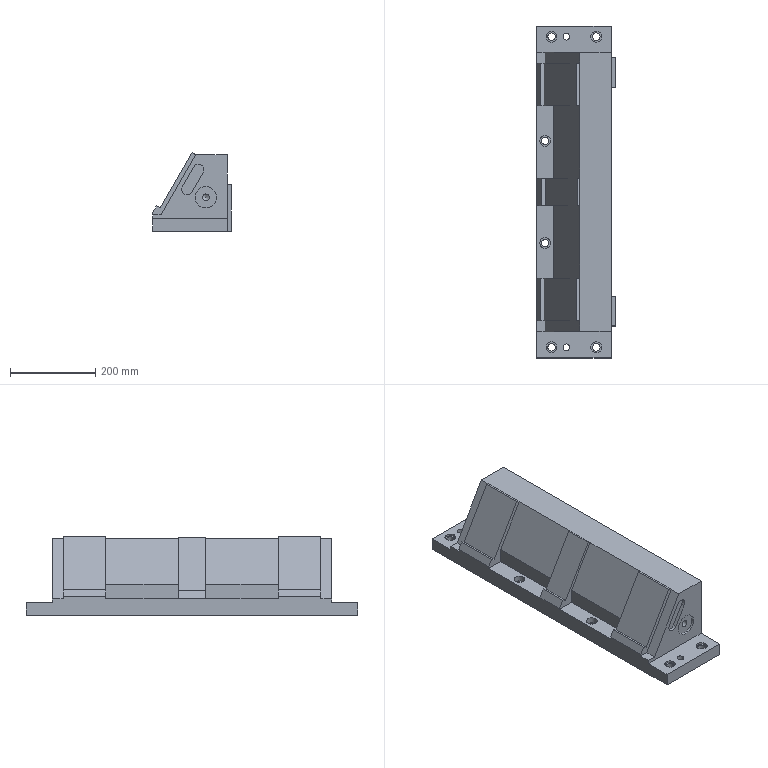Part | NX | features solid 2 | 1 solid | 94 faces | box 185 x 780 x 184.958 mm | volume 12906124 mm3 | plane 70 | cylinder 22 | cone 2 | commonest cylinder face diameters 16 x4 17.5 x4 25 x4 25.5 x4 18 x2 26 x2